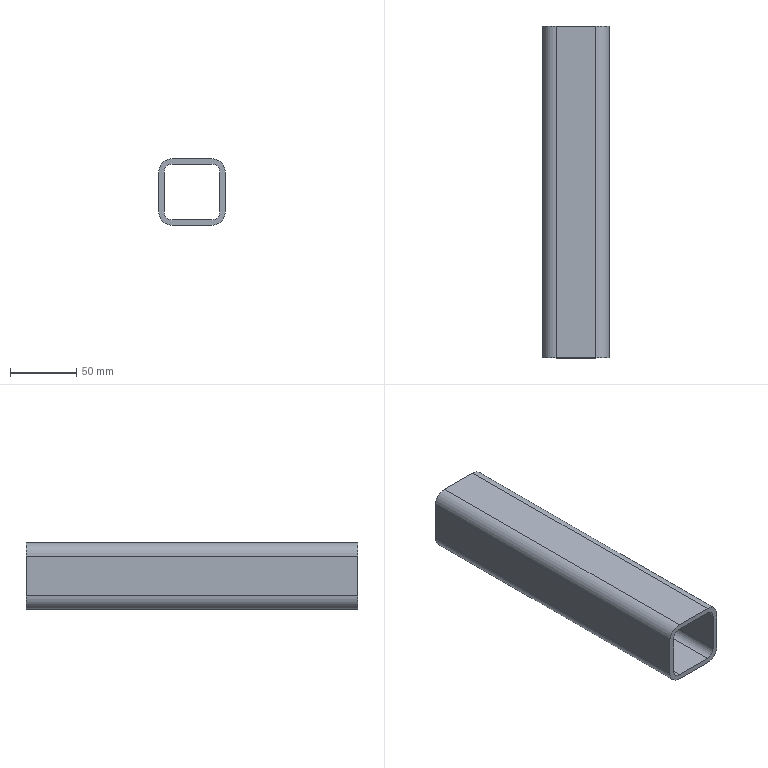Part | SolidWorks | features Extrusion 1 | 1 solid | 18 faces | box 50 x 250 x 50 mm | volume 170265 mm3 | plane 10 | cylinder 8 | commonest cylinder face diameters 12 x4 20 x4
STEP:
#1=CARTESIAN_POINT('',(15.,250.,25.));
#2=VERTEX_POINT('',#1);
#3=CARTESIAN_POINT('',(25.,250.,15.));
#4=VERTEX_POINT('',#3);
#5=CARTESIAN_POINT('',(15.,250.,15.));
#6=DIRECTION('',(0.,1.,0.));
#7=DIRECTION('',(0.,0.,1.));
#8=AXIS2_PLACEMENT_3D('',#5,#6,#7);
#9=CIRCLE('',#8,10.);
#10=EDGE_CURVE('',#2,#4,#9,.T.);
#11=ORIENTED_EDGE('',*,*,#10,.T.);
#12=CARTESIAN_POINT('',(25.,250.,-15.));
#13=VERTEX_POINT('',#12);
#14=CARTESIAN_POINT('',(25.,250.,15.));
#15=DIRECTION('',(0.,0.,-1.));
#16=VECTOR('',#15,1000.);
#17=LINE('',#14,#16);
#18=EDGE_CURVE('',#4,#13,#17,.T.);
#19=ORIENTED_EDGE('',*,*,#18,.T.);
#20=CARTESIAN_POINT('',(15.,250.,-25.));
#21=VERTEX_POINT('',#20);
#22=CARTESIAN_POINT('',(15.,250.,-15.));
#23=DIRECTION('',(0.,1.,0.));
#24=DIRECTION('',(0.,0.,-1.));
#25=AXIS2_PLACEMENT_3D('',#22,#23,#24);
#26=CIRCLE('',#25,10.);
#27=EDGE_CURVE('',#13,#21,#26,.T.);
#28=ORIENTED_EDGE('',*,*,#27,.T.);
#29=CARTESIAN_POINT('',(-15.,250.,-25.));
#30=VERTEX_POINT('',#29);
#31=CARTESIAN_POINT('',(-15.,250.,-25.));
#32=DIRECTION('',(-1.,0.,0.));
#33=VECTOR('',#32,1000.);
#34=LINE('',#31,#33);
#35=EDGE_CURVE('',#21,#30,#34,.T.);
#36=ORIENTED_EDGE('',*,*,#35,.T.);
#37=CARTESIAN_POINT('',(-25.,250.,-15.));
#38=VERTEX_POINT('',#37);
#39=CARTESIAN_POINT('',(-15.,250.,-15.));
#40=DIRECTION('',(0.,1.,0.));
#41=DIRECTION('',(0.,0.,-1.));
#42=AXIS2_PLACEMENT_3D('',#39,#40,#41);
#43=CIRCLE('',#42,10.);
#44=EDGE_CURVE('',#30,#38,#43,.T.);
#45=ORIENTED_EDGE('',*,*,#44,.T.);
#46=CARTESIAN_POINT('',(-25.,250.,15.));
#47=VERTEX_POINT('',#46);
#48=CARTESIAN_POINT('',(-25.,250.,15.));
#49=DIRECTION('',(0.,0.,1.));
#50=VECTOR('',#49,1000.);
#51=LINE('',#48,#50);
#52=EDGE_CURVE('',#38,#47,#51,.T.);
#53=ORIENTED_EDGE('',*,*,#52,.T.);
#54=CARTESIAN_POINT('',(-15.,250.,25.));
#55=VERTEX_POINT('',#54);
#56=CARTESIAN_POINT('',(-15.,250.,15.));
#57=DIRECTION('',(0.,1.,0.));
#58=DIRECTION('',(0.,0.,-1.));
#59=AXIS2_PLACEMENT_3D('',#56,#57,#58);
#60=CIRCLE('',#59,10.);
#61=EDGE_CURVE('',#47,#55,#60,.T.);
#62=ORIENTED_EDGE('',*,*,#61,.T.);
#63=CARTESIAN_POINT('',(-15.,250.,25.));
#64=DIRECTION('',(1.,0.,0.));
#65=VECTOR('',#64,1000.);
#66=LINE('',#63,#65);
#67=EDGE_CURVE('',#55,#2,#66,.T.);
#68=ORIENTED_EDGE('',*,*,#67,.T.);
#69=EDGE_LOOP('',(#11,#19,#28,#36,#45,#53,#62,#68));
#70=FACE_OUTER_BOUND('',#69,.T.);
#71=CARTESIAN_POINT('',(-21.,250.,-15.));
#72=VERTEX_POINT('',#71);
#73=CARTESIAN_POINT('',(-21.,250.,15.));
#74=VERTEX_POINT('',#73);
#75=CARTESIAN_POINT('',(-21.,250.,15.));
#76=DIRECTION('',(0.,0.,1.));
#77=VECTOR('',#76,1000.);
#78=LINE('',#75,#77);
#79=EDGE_CURVE('',#72,#74,#78,.T.);
#80=ORIENTED_EDGE('',*,*,#79,.F.);
#81=CARTESIAN_POINT('',(-15.,250.,-21.));
#82=VERTEX_POINT('',#81);
#83=CARTESIAN_POINT('',(-15.,250.,-15.));
#84=DIRECTION('',(0.,1.,0.));
#85=DIRECTION('',(0.,0.,-1.));
#86=AXIS2_PLACEMENT_3D('',#83,#84,#85);
#87=CIRCLE('',#86,6.);
#88=EDGE_CURVE('',#82,#72,#87,.T.);
#89=ORIENTED_EDGE('',*,*,#88,.F.);
#90=CARTESIAN_POINT('',(15.,250.,-21.));
#91=VERTEX_POINT('',#90);
#92=CARTESIAN_POINT('',(-15.,250.,-21.));
#93=DIRECTION('',(-1.,0.,0.));
#94=VECTOR('',#93,1000.);
#95=LINE('',#92,#94);
#96=EDGE_CURVE('',#91,#82,#95,.T.);
#97=ORIENTED_EDGE('',*,*,#96,.F.);
#98=CARTESIAN_POINT('',(21.,250.,-15.));
#99=VERTEX_POINT('',#98);
#100=CARTESIAN_POINT('',(15.,250.,-15.));
#101=DIRECTION('',(0.,1.,0.));
#102=DIRECTION('',(0.,0.,-1.));
#103=AXIS2_PLACEMENT_3D('',#100,#101,#102);
#104=CIRCLE('',#103,6.);
#105=EDGE_CURVE('',#99,#91,#104,.T.);
#106=ORIENTED_EDGE('',*,*,#105,.F.);
#107=CARTESIAN_POINT('',(21.,250.,15.));
#108=VERTEX_POINT('',#107);
#109=CARTESIAN_POINT('',(21.,250.,15.));
#110=DIRECTION('',(0.,0.,-1.));
#111=VECTOR('',#110,1000.);
#112=LINE('',#109,#111);
#113=EDGE_CURVE('',#108,#99,#112,.T.);
#114=ORIENTED_EDGE('',*,*,#113,.F.);
#115=CARTESIAN_POINT('',(15.,250.,21.));
#116=VERTEX_POINT('',#115);
#117=CARTESIAN_POINT('',(15.,250.,15.));
#118=DIRECTION('',(0.,1.,0.));
#119=DIRECTION('',(0.,0.,1.));
#120=AXIS2_PLACEMENT_3D('',#117,#118,#119);
#121=CIRCLE('',#120,6.);
#122=EDGE_CURVE('',#116,#108,#121,.T.);
#123=ORIENTED_EDGE('',*,*,#122,.F.);
#124=CARTESIAN_POINT('',(-15.,250.,21.));
#125=VERTEX_POINT('',#124);
#126=CARTESIAN_POINT('',(-15.,250.,21.));
#127=DIRECTION('',(1.,0.,0.));
#128=VECTOR('',#127,1000.);
#129=LINE('',#126,#128);
#130=EDGE_CURVE('',#125,#116,#129,.T.);
#131=ORIENTED_EDGE('',*,*,#130,.F.);
#132=CARTESIAN_POINT('',(-15.,250.,15.));
#133=DIRECTION('',(0.,1.,0.));
#134=DIRECTION('',(0.,0.,-1.));
#135=AXIS2_PLACEMENT_3D('',#132,#133,#134);
#136=CIRCLE('',#135,6.);
#137=EDGE_CURVE('',#74,#125,#136,.T.);
#138=ORIENTED_EDGE('',*,*,#137,.F.);
#139=EDGE_LOOP('',(#80,#89,#97,#106,#114,#123,#131,#138));
#140=FACE_BOUND('',#139,.T.);
#141=CARTESIAN_POINT('',(15.,250.,15.));
#142=DIRECTION('',(0.,1.,0.));
#143=DIRECTION('',(0.,0.,1.));
#144=AXIS2_PLACEMENT_3D('',#141,#142,#143);
#145=PLANE('',#144);
#146=ADVANCED_FACE('',(#70,#140),#145,.T.);
#147=CARTESIAN_POINT('',(15.,0.,25.));
#148=VERTEX_POINT('',#147);
#149=CARTESIAN_POINT('',(25.,0.,15.));
#150=VERTEX_POINT('',#149);
#151=CARTESIAN_POINT('',(15.,0.,15.));
#152=DIRECTION('',(0.,1.,0.));
#153=DIRECTION('',(0.,0.,1.));
#154=AXIS2_PLACEMENT_3D('',#151,#152,#153);
#155=CIRCLE('',#154,10.);
#156=EDGE_CURVE('',#148,#150,#155,.T.);
#157=ORIENTED_EDGE('',*,*,#156,.F.);
#158=CARTESIAN_POINT('',(-15.,0.,25.));
#159=VERTEX_POINT('',#158);
#160=CARTESIAN_POINT('',(-15.,0.,25.));
#161=DIRECTION('',(1.,0.,0.));
#162=VECTOR('',#161,1000.);
#163=LINE('',#160,#162);
#164=EDGE_CURVE('',#159,#148,#163,.T.);
#165=ORIENTED_EDGE('',*,*,#164,.F.);
#166=CARTESIAN_POINT('',(-25.,0.,15.));
#167=VERTEX_POINT('',#166);
#168=CARTESIAN_POINT('',(-15.,0.,15.));
#169=DIRECTION('',(0.,1.,0.));
#170=DIRECTION('',(0.,0.,-1.));
#171=AXIS2_PLACEMENT_3D('',#168,#169,#170);
#172=CIRCLE('',#171,10.);
#173=EDGE_CURVE('',#167,#159,#172,.T.);
#174=ORIENTED_EDGE('',*,*,#173,.F.);
#175=CARTESIAN_POINT('',(-25.,0.,-15.));
#176=VERTEX_POINT('',#175);
#177=CARTESIAN_POINT('',(-25.,0.,15.));
#178=DIRECTION('',(0.,0.,1.));
#179=VECTOR('',#178,1000.);
#180=LINE('',#177,#179);
#181=EDGE_CURVE('',#176,#167,#180,.T.);
#182=ORIENTED_EDGE('',*,*,#181,.F.);
#183=CARTESIAN_POINT('',(-15.,0.,-25.));
#184=VERTEX_POINT('',#183);
#185=CARTESIAN_POINT('',(-15.,0.,-15.));
#186=DIRECTION('',(0.,1.,0.));
#187=DIRECTION('',(0.,0.,-1.));
#188=AXIS2_PLACEMENT_3D('',#185,#186,#187);
#189=CIRCLE('',#188,10.);
#190=EDGE_CURVE('',#184,#176,#189,.T.);
#191=ORIENTED_EDGE('',*,*,#190,.F.);
#192=CARTESIAN_POINT('',(15.,0.,-25.));
#193=VERTEX_POINT('',#192);
#194=CARTESIAN_POINT('',(-15.,0.,-25.));
#195=DIRECTION('',(-1.,0.,0.));
#196=VECTOR('',#195,1000.);
#197=LINE('',#194,#196);
#198=EDGE_CURVE('',#193,#184,#197,.T.);
#199=ORIENTED_EDGE('',*,*,#198,.F.);
#200=CARTESIAN_POINT('',(25.,0.,-15.));
#201=VERTEX_POINT('',#200);
#202=CARTESIAN_POINT('',(15.,0.,-15.));
#203=DIRECTION('',(0.,1.,0.));
#204=DIRECTION('',(0.,0.,-1.));
#205=AXIS2_PLACEMENT_3D('',#202,#203,#204);
#206=CIRCLE('',#205,10.);
#207=EDGE_CURVE('',#201,#193,#206,.T.);
#208=ORIENTED_EDGE('',*,*,#207,.F.);
#209=CARTESIAN_POINT('',(25.,0.,15.));
#210=DIRECTION('',(0.,0.,-1.));
#211=VECTOR('',#210,1000.);
#212=LINE('',#209,#211);
#213=EDGE_CURVE('',#150,#201,#212,.T.);
#214=ORIENTED_EDGE('',*,*,#213,.F.);
#215=EDGE_LOOP('',(#157,#165,#174,#182,#191,#199,#208,#214));
#216=FACE_OUTER_BOUND('',#215,.T.);
#217=CARTESIAN_POINT('',(-15.,0.,-21.));
#218=VERTEX_POINT('',#217);
#219=CARTESIAN_POINT('',(-21.,0.,-15.));
#220=VERTEX_POINT('',#219);
#221=CARTESIAN_POINT('',(-15.,0.,-15.));
#222=DIRECTION('',(0.,1.,0.));
#223=DIRECTION('',(0.,0.,-1.));
#224=AXIS2_PLACEMENT_3D('',#221,#222,#223);
#225=CIRCLE('',#224,6.);
#226=EDGE_CURVE('',#218,#220,#225,.T.);
#227=ORIENTED_EDGE('',*,*,#226,.T.);
#228=CARTESIAN_POINT('',(-21.,0.,15.));
#229=VERTEX_POINT('',#228);
#230=CARTESIAN_POINT('',(-21.,0.,15.));
#231=DIRECTION('',(0.,0.,1.));
#232=VECTOR('',#231,1000.);
#233=LINE('',#230,#232);
#234=EDGE_CURVE('',#220,#229,#233,.T.);
#235=ORIENTED_EDGE('',*,*,#234,.T.);
#236=CARTESIAN_POINT('',(-15.,0.,21.));
#237=VERTEX_POINT('',#236);
#238=CARTESIAN_POINT('',(-15.,0.,15.));
#239=DIRECTION('',(0.,1.,0.));
#240=DIRECTION('',(0.,0.,-1.));
#241=AXIS2_PLACEMENT_3D('',#238,#239,#240);
#242=CIRCLE('',#241,6.);
#243=EDGE_CURVE('',#229,#237,#242,.T.);
#244=ORIENTED_EDGE('',*,*,#243,.T.);
#245=CARTESIAN_POINT('',(15.,0.,21.));
#246=VERTEX_POINT('',#245);
#247=CARTESIAN_POINT('',(-15.,0.,21.));
#248=DIRECTION('',(1.,0.,0.));
#249=VECTOR('',#248,1000.);
#250=LINE('',#247,#249);
#251=EDGE_CURVE('',#237,#246,#250,.T.);
#252=ORIENTED_EDGE('',*,*,#251,.T.);
#253=CARTESIAN_POINT('',(21.,0.,15.));
#254=VERTEX_POINT('',#253);
#255=CARTESIAN_POINT('',(15.,0.,15.));
#256=DIRECTION('',(0.,1.,0.));
#257=DIRECTION('',(0.,0.,1.));
#258=AXIS2_PLACEMENT_3D('',#255,#256,#257);
#259=CIRCLE('',#258,6.);
#260=EDGE_CURVE('',#246,#254,#259,.T.);
#261=ORIENTED_EDGE('',*,*,#260,.T.);
#262=CARTESIAN_POINT('',(21.,0.,-15.));
#263=VERTEX_POINT('',#262);
#264=CARTESIAN_POINT('',(21.,0.,15.));
#265=DIRECTION('',(0.,0.,-1.));
#266=VECTOR('',#265,1000.);
#267=LINE('',#264,#266);
#268=EDGE_CURVE('',#254,#263,#267,.T.);
#269=ORIENTED_EDGE('',*,*,#268,.T.);
#270=CARTESIAN_POINT('',(15.,0.,-21.));
#271=VERTEX_POINT('',#270);
#272=CARTESIAN_POINT('',(15.,0.,-15.));
#273=DIRECTION('',(0.,1.,0.));
#274=DIRECTION('',(0.,0.,-1.));
#275=AXIS2_PLACEMENT_3D('',#272,#273,#274);
#276=CIRCLE('',#275,6.);
#277=EDGE_CURVE('',#263,#271,#276,.T.);
#278=ORIENTED_EDGE('',*,*,#277,.T.);
#279=CARTESIAN_POINT('',(-15.,0.,-21.));
#280=DIRECTION('',(-1.,0.,0.));
#281=VECTOR('',#280,1000.);
#282=LINE('',#279,#281);
#283=EDGE_CURVE('',#271,#218,#282,.T.);
#284=ORIENTED_EDGE('',*,*,#283,.T.);
#285=EDGE_LOOP('',(#227,#235,#244,#252,#261,#269,#278,#284));
#286=FACE_BOUND('',#285,.T.);
#287=CARTESIAN_POINT('',(15.,0.,15.));
#288=DIRECTION('',(0.,1.,0.));
#289=DIRECTION('',(0.,0.,1.));
#290=AXIS2_PLACEMENT_3D('',#287,#288,#289);
#291=PLANE('',#290);
#292=ADVANCED_FACE('',(#216,#286),#291,.F.);
#293=ORIENTED_EDGE('',*,*,#156,.T.);
#294=CARTESIAN_POINT('',(25.,250.,15.));
#295=DIRECTION('',(0.,-1.,0.));
#296=VECTOR('',#295,1000.);
#297=LINE('',#294,#296);
#298=EDGE_CURVE('',#4,#150,#297,.T.);
#299=ORIENTED_EDGE('',*,*,#298,.F.);
#300=ORIENTED_EDGE('',*,*,#10,.F.);
#301=CARTESIAN_POINT('',(15.,250.,25.));
#302=DIRECTION('',(0.,-1.,0.));
#303=VECTOR('',#302,1000.);
#304=LINE('',#301,#303);
#305=EDGE_CURVE('',#2,#148,#304,.T.);
#306=ORIENTED_EDGE('',*,*,#305,.T.);
#307=EDGE_LOOP('',(#293,#299,#300,#306));
#308=FACE_OUTER_BOUND('',#307,.T.);
#309=CARTESIAN_POINT('',(15.,250.,15.));
#310=DIRECTION('',(0.,-1.,0.));
#311=DIRECTION('',(0.,0.,-1.));
#312=AXIS2_PLACEMENT_3D('',#309,#310,#311);
#313=CYLINDRICAL_SURFACE('',#312,10.);
#314=ADVANCED_FACE('',(#308),#313,.T.);
#315=ORIENTED_EDGE('',*,*,#213,.T.);
#316=CARTESIAN_POINT('',(25.,250.,-15.));
#317=DIRECTION('',(0.,-1.,0.));
#318=VECTOR('',#317,1000.);
#319=LINE('',#316,#318);
#320=EDGE_CURVE('',#13,#201,#319,.T.);
#321=ORIENTED_EDGE('',*,*,#320,.F.);
#322=ORIENTED_EDGE('',*,*,#18,.F.);
#323=ORIENTED_EDGE('',*,*,#298,.T.);
#324=EDGE_LOOP('',(#315,#321,#322,#323));
#325=FACE_OUTER_BOUND('',#324,.T.);
#326=CARTESIAN_POINT('',(25.,250.,15.));
#327=DIRECTION('',(-1.,0.,0.));
#328=DIRECTION('',(0.,0.,1.));
#329=AXIS2_PLACEMENT_3D('',#326,#327,#328);
#330=PLANE('',#329);
#331=ADVANCED_FACE('',(#325),#330,.F.);
#332=ORIENTED_EDGE('',*,*,#207,.T.);
#333=CARTESIAN_POINT('',(15.,250.,-25.));
#334=DIRECTION('',(0.,-1.,0.));
#335=VECTOR('',#334,1000.);
#336=LINE('',#333,#335);
#337=EDGE_CURVE('',#21,#193,#336,.T.);
#338=ORIENTED_EDGE('',*,*,#337,.F.);
#339=ORIENTED_EDGE('',*,*,#27,.F.);
#340=ORIENTED_EDGE('',*,*,#320,.T.);
#341=EDGE_LOOP('',(#332,#338,#339,#340));
#342=FACE_OUTER_BOUND('',#341,.T.);
#343=CARTESIAN_POINT('',(15.,250.,-15.));
#344=DIRECTION('',(0.,-1.,0.));
#345=DIRECTION('',(0.,0.,-1.));
#346=AXIS2_PLACEMENT_3D('',#343,#344,#345);
#347=CYLINDRICAL_SURFACE('',#346,10.);
#348=ADVANCED_FACE('',(#342),#347,.T.);
#349=ORIENTED_EDGE('',*,*,#198,.T.);
#350=CARTESIAN_POINT('',(-15.,250.,-25.));
#351=DIRECTION('',(0.,-1.,0.));
#352=VECTOR('',#351,1000.);
#353=LINE('',#350,#352);
#354=EDGE_CURVE('',#30,#184,#353,.T.);
#355=ORIENTED_EDGE('',*,*,#354,.F.);
#356=ORIENTED_EDGE('',*,*,#35,.F.);
#357=ORIENTED_EDGE('',*,*,#337,.T.);
#358=EDGE_LOOP('',(#349,#355,#356,#357));
#359=FACE_OUTER_BOUND('',#358,.T.);
#360=CARTESIAN_POINT('',(-15.,250.,-25.));
#361=DIRECTION('',(0.,0.,1.));
#362=DIRECTION('',(1.,0.,0.));
#363=AXIS2_PLACEMENT_3D('',#360,#361,#362);
#364=PLANE('',#363);
#365=ADVANCED_FACE('',(#359),#364,.F.);
#366=ORIENTED_EDGE('',*,*,#190,.T.);
#367=CARTESIAN_POINT('',(-25.,250.,-15.));
#368=DIRECTION('',(0.,-1.,0.));
#369=VECTOR('',#368,1000.);
#370=LINE('',#367,#369);
#371=EDGE_CURVE('',#38,#176,#370,.T.);
#372=ORIENTED_EDGE('',*,*,#371,.F.);
#373=ORIENTED_EDGE('',*,*,#44,.F.);
#374=ORIENTED_EDGE('',*,*,#354,.T.);
#375=EDGE_LOOP('',(#366,#372,#373,#374));
#376=FACE_OUTER_BOUND('',#375,.T.);
#377=CARTESIAN_POINT('',(-15.,250.,-15.));
#378=DIRECTION('',(0.,-1.,0.));
#379=DIRECTION('',(0.,0.,-1.));
#380=AXIS2_PLACEMENT_3D('',#377,#378,#379);
#381=CYLINDRICAL_SURFACE('',#380,10.);
#382=ADVANCED_FACE('',(#376),#381,.T.);
#383=ORIENTED_EDGE('',*,*,#181,.T.);
#384=CARTESIAN_POINT('',(-25.,250.,15.));
#385=DIRECTION('',(0.,-1.,0.));
#386=VECTOR('',#385,1000.);
#387=LINE('',#384,#386);
#388=EDGE_CURVE('',#47,#167,#387,.T.);
#389=ORIENTED_EDGE('',*,*,#388,.F.);
#390=ORIENTED_EDGE('',*,*,#52,.F.);
#391=ORIENTED_EDGE('',*,*,#371,.T.);
#392=EDGE_LOOP('',(#383,#389,#390,#391));
#393=FACE_OUTER_BOUND('',#392,.T.);
#394=CARTESIAN_POINT('',(-25.,250.,15.));
#395=DIRECTION('',(1.,0.,0.));
#396=DIRECTION('',(0.,0.,-1.));
#397=AXIS2_PLACEMENT_3D('',#394,#395,#396);
#398=PLANE('',#397);
#399=ADVANCED_FACE('',(#393),#398,.F.);
#400=ORIENTED_EDGE('',*,*,#173,.T.);
#401=CARTESIAN_POINT('',(-15.,250.,25.));
#402=DIRECTION('',(0.,-1.,0.));
#403=VECTOR('',#402,1000.);
#404=LINE('',#401,#403);
#405=EDGE_CURVE('',#55,#159,#404,.T.);
#406=ORIENTED_EDGE('',*,*,#405,.F.);
#407=ORIENTED_EDGE('',*,*,#61,.F.);
#408=ORIENTED_EDGE('',*,*,#388,.T.);
#409=EDGE_LOOP('',(#400,#406,#407,#408));
#410=FACE_OUTER_BOUND('',#409,.T.);
#411=CARTESIAN_POINT('',(-15.,250.,15.));
#412=DIRECTION('',(0.,-1.,0.));
#413=DIRECTION('',(0.,0.,-1.));
#414=AXIS2_PLACEMENT_3D('',#411,#412,#413);
#415=CYLINDRICAL_SURFACE('',#414,10.);
#416=ADVANCED_FACE('',(#410),#415,.T.);
#417=ORIENTED_EDGE('',*,*,#164,.T.);
#418=ORIENTED_EDGE('',*,*,#305,.F.);
#419=ORIENTED_EDGE('',*,*,#67,.F.);
#420=ORIENTED_EDGE('',*,*,#405,.T.);
#421=EDGE_LOOP('',(#417,#418,#419,#420));
#422=FACE_OUTER_BOUND('',#421,.T.);
#423=CARTESIAN_POINT('',(-15.,250.,25.));
#424=DIRECTION('',(0.,0.,-1.));
#425=DIRECTION('',(-1.,0.,0.));
#426=AXIS2_PLACEMENT_3D('',#423,#424,#425);
#427=PLANE('',#426);
#428=ADVANCED_FACE('',(#422),#427,.F.);
#429=ORIENTED_EDGE('',*,*,#226,.F.);
#430=CARTESIAN_POINT('',(-15.,250.,-21.));
#431=DIRECTION('',(0.,-1.,0.));
#432=VECTOR('',#431,1000.);
#433=LINE('',#430,#432);
#434=EDGE_CURVE('',#82,#218,#433,.T.);
#435=ORIENTED_EDGE('',*,*,#434,.F.);
#436=ORIENTED_EDGE('',*,*,#88,.T.);
#437=CARTESIAN_POINT('',(-21.,250.,-15.));
#438=DIRECTION('',(0.,-1.,0.));
#439=VECTOR('',#438,1000.);
#440=LINE('',#437,#439);
#441=EDGE_CURVE('',#72,#220,#440,.T.);
#442=ORIENTED_EDGE('',*,*,#441,.T.);
#443=EDGE_LOOP('',(#429,#435,#436,#442));
#444=FACE_OUTER_BOUND('',#443,.T.);
#445=CARTESIAN_POINT('',(-15.,250.,-15.));
#446=DIRECTION('',(0.,-1.,0.));
#447=DIRECTION('',(0.,0.,-1.));
#448=AXIS2_PLACEMENT_3D('',#445,#446,#447);
#449=CYLINDRICAL_SURFACE('',#448,6.);
#450=ADVANCED_FACE('',(#444),#449,.F.);
#451=ORIENTED_EDGE('',*,*,#234,.F.);
#452=ORIENTED_EDGE('',*,*,#441,.F.);
#453=ORIENTED_EDGE('',*,*,#79,.T.);
#454=CARTESIAN_POINT('',(-21.,250.,15.));
#455=DIRECTION('',(0.,-1.,0.));
#456=VECTOR('',#455,1000.);
#457=LINE('',#454,#456);
#458=EDGE_CURVE('',#74,#229,#457,.T.);
#459=ORIENTED_EDGE('',*,*,#458,.T.);
#460=EDGE_LOOP('',(#451,#452,#453,#459));
#461=FACE_OUTER_BOUND('',#460,.T.);
#462=CARTESIAN_POINT('',(-21.,250.,15.));
#463=DIRECTION('',(1.,0.,0.));
#464=DIRECTION('',(0.,0.,-1.));
#465=AXIS2_PLACEMENT_3D('',#462,#463,#464);
#466=PLANE('',#465);
#467=ADVANCED_FACE('',(#461),#466,.T.);
#468=ORIENTED_EDGE('',*,*,#243,.F.);
#469=ORIENTED_EDGE('',*,*,#458,.F.);
#470=ORIENTED_EDGE('',*,*,#137,.T.);
#471=CARTESIAN_POINT('',(-15.,250.,21.));
#472=DIRECTION('',(0.,-1.,0.));
#473=VECTOR('',#472,1000.);
#474=LINE('',#471,#473);
#475=EDGE_CURVE('',#125,#237,#474,.T.);
#476=ORIENTED_EDGE('',*,*,#475,.T.);
#477=EDGE_LOOP('',(#468,#469,#470,#476));
#478=FACE_OUTER_BOUND('',#477,.T.);
#479=CARTESIAN_POINT('',(-15.,250.,15.));
#480=DIRECTION('',(0.,-1.,0.));
#481=DIRECTION('',(0.,0.,-1.));
#482=AXIS2_PLACEMENT_3D('',#479,#480,#481);
#483=CYLINDRICAL_SURFACE('',#482,6.);
#484=ADVANCED_FACE('',(#478),#483,.F.);
#485=ORIENTED_EDGE('',*,*,#251,.F.);
#486=ORIENTED_EDGE('',*,*,#475,.F.);
#487=ORIENTED_EDGE('',*,*,#130,.T.);
#488=CARTESIAN_POINT('',(15.,250.,21.));
#489=DIRECTION('',(0.,-1.,0.));
#490=VECTOR('',#489,1000.);
#491=LINE('',#488,#490);
#492=EDGE_CURVE('',#116,#246,#491,.T.);
#493=ORIENTED_EDGE('',*,*,#492,.T.);
#494=EDGE_LOOP('',(#485,#486,#487,#493));
#495=FACE_OUTER_BOUND('',#494,.T.);
#496=CARTESIAN_POINT('',(-15.,250.,21.));
#497=DIRECTION('',(0.,0.,-1.));
#498=DIRECTION('',(-1.,0.,0.));
#499=AXIS2_PLACEMENT_3D('',#496,#497,#498);
#500=PLANE('',#499);
#501=ADVANCED_FACE('',(#495),#500,.T.);
#502=ORIENTED_EDGE('',*,*,#260,.F.);
#503=ORIENTED_EDGE('',*,*,#492,.F.);
#504=ORIENTED_EDGE('',*,*,#122,.T.);
#505=CARTESIAN_POINT('',(21.,250.,15.));
#506=DIRECTION('',(0.,-1.,0.));
#507=VECTOR('',#506,1000.);
#508=LINE('',#505,#507);
#509=EDGE_CURVE('',#108,#254,#508,.T.);
#510=ORIENTED_EDGE('',*,*,#509,.T.);
#511=EDGE_LOOP('',(#502,#503,#504,#510));
#512=FACE_OUTER_BOUND('',#511,.T.);
#513=CARTESIAN_POINT('',(15.,250.,15.));
#514=DIRECTION('',(0.,-1.,0.));
#515=DIRECTION('',(0.,0.,-1.));
#516=AXIS2_PLACEMENT_3D('',#513,#514,#515);
#517=CYLINDRICAL_SURFACE('',#516,6.);
#518=ADVANCED_FACE('',(#512),#517,.F.);
#519=ORIENTED_EDGE('',*,*,#268,.F.);
#520=ORIENTED_EDGE('',*,*,#509,.F.);
#521=ORIENTED_EDGE('',*,*,#113,.T.);
#522=CARTESIAN_POINT('',(21.,250.,-15.));
#523=DIRECTION('',(0.,-1.,0.));
#524=VECTOR('',#523,1000.);
#525=LINE('',#522,#524);
#526=EDGE_CURVE('',#99,#263,#525,.T.);
#527=ORIENTED_EDGE('',*,*,#526,.T.);
#528=EDGE_LOOP('',(#519,#520,#521,#527));
#529=FACE_OUTER_BOUND('',#528,.T.);
#530=CARTESIAN_POINT('',(21.,250.,15.));
#531=DIRECTION('',(-1.,0.,0.));
#532=DIRECTION('',(0.,0.,1.));
#533=AXIS2_PLACEMENT_3D('',#530,#531,#532);
#534=PLANE('',#533);
#535=ADVANCED_FACE('',(#529),#534,.T.);
#536=ORIENTED_EDGE('',*,*,#277,.F.);
#537=ORIENTED_EDGE('',*,*,#526,.F.);
#538=ORIENTED_EDGE('',*,*,#105,.T.);
#539=CARTESIAN_POINT('',(15.,250.,-21.));
#540=DIRECTION('',(0.,-1.,0.));
#541=VECTOR('',#540,1000.);
#542=LINE('',#539,#541);
#543=EDGE_CURVE('',#91,#271,#542,.T.);
#544=ORIENTED_EDGE('',*,*,#543,.T.);
#545=EDGE_LOOP('',(#536,#537,#538,#544));
#546=FACE_OUTER_BOUND('',#545,.T.);
#547=CARTESIAN_POINT('',(15.,250.,-15.));
#548=DIRECTION('',(0.,-1.,0.));
#549=DIRECTION('',(0.,0.,-1.));
#550=AXIS2_PLACEMENT_3D('',#547,#548,#549);
#551=CYLINDRICAL_SURFACE('',#550,6.);
#552=ADVANCED_FACE('',(#546),#551,.F.);
#553=ORIENTED_EDGE('',*,*,#283,.F.);
#554=ORIENTED_EDGE('',*,*,#543,.F.);
#555=ORIENTED_EDGE('',*,*,#96,.T.);
#556=ORIENTED_EDGE('',*,*,#434,.T.);
#557=EDGE_LOOP('',(#553,#554,#555,#556));
#558=FACE_OUTER_BOUND('',#557,.T.);
#559=CARTESIAN_POINT('',(-15.,250.,-21.));
#560=DIRECTION('',(0.,0.,1.));
#561=DIRECTION('',(1.,0.,0.));
#562=AXIS2_PLACEMENT_3D('',#559,#560,#561);
#563=PLANE('',#562);
#564=ADVANCED_FACE('',(#558),#563,.T.);
#565=CLOSED_SHELL('',(#146,#292,#314,#331,#348,#365,#382,#399,#416,#428,#450,#467,#484,#501,#518,#535,#552,#564));
#566=MANIFOLD_SOLID_BREP('',#565);
#567=CARTESIAN_POINT('',(0.,0.,0.));
#568=DIRECTION('',(0.,0.,1.));
#569=DIRECTION('',(1.,0.,0.));
#570=AXIS2_PLACEMENT_3D('',#567,#568,#569);
#571=(LENGTH_UNIT()NAMED_UNIT(*)SI_UNIT(.MILLI.,.METRE.));
#572=UNCERTAINTY_MEASURE_WITH_UNIT(LENGTH_MEASURE(0.00001),#571,'','');
#573=(NAMED_UNIT(*)PLANE_ANGLE_UNIT()SI_UNIT($,.RADIAN.));
#574=(NAMED_UNIT(*)SI_UNIT($,.STERADIAN.)SOLID_ANGLE_UNIT());
#575=(GEOMETRIC_REPRESENTATION_CONTEXT(3)GLOBAL_UNCERTAINTY_ASSIGNED_CONTEXT((#572))GLOBAL_UNIT_ASSIGNED_CONTEXT((#571,#573,#574))REPRESENTATION_CONTEXT('',''));
#576=ADVANCED_BREP_SHAPE_REPRESENTATION('',(#566,#570),#575);